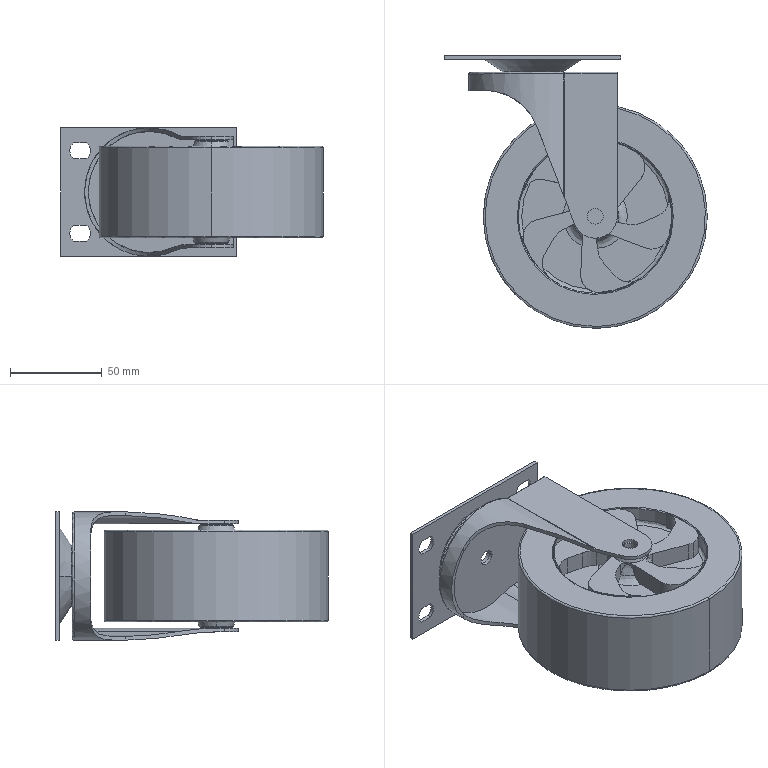Part | SolidWorks | features BaseBody 10, CombineBodies 2 | 3 solids | 233 faces | box 143 x 148.5 x 70 mm | volume 563559 mm3 | cylinder 102 | plane 74 | spline 37 | cone 20 | commonest cylinder face diameters 19.115 x13 8.5 x12 11.2 x12 11.664 x12 18.927 x12 26.97 x11